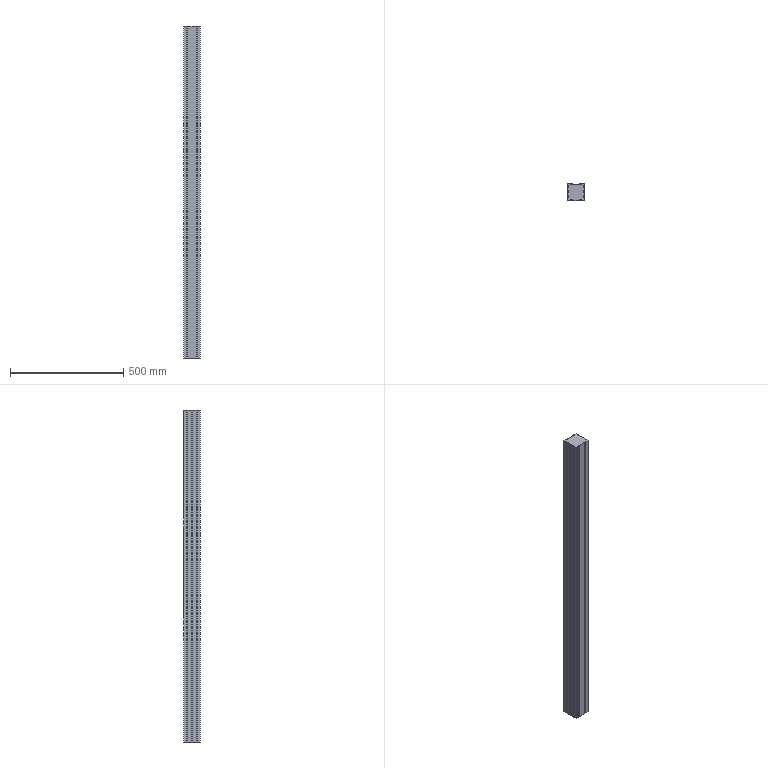Part | SolidWorks | features ICE 3, Extrusion 1, MirrorPattern 1 | 1 solid | 74 faces | box 75 x 75 x 1465 mm | volume 7717503 mm3 | plane 74